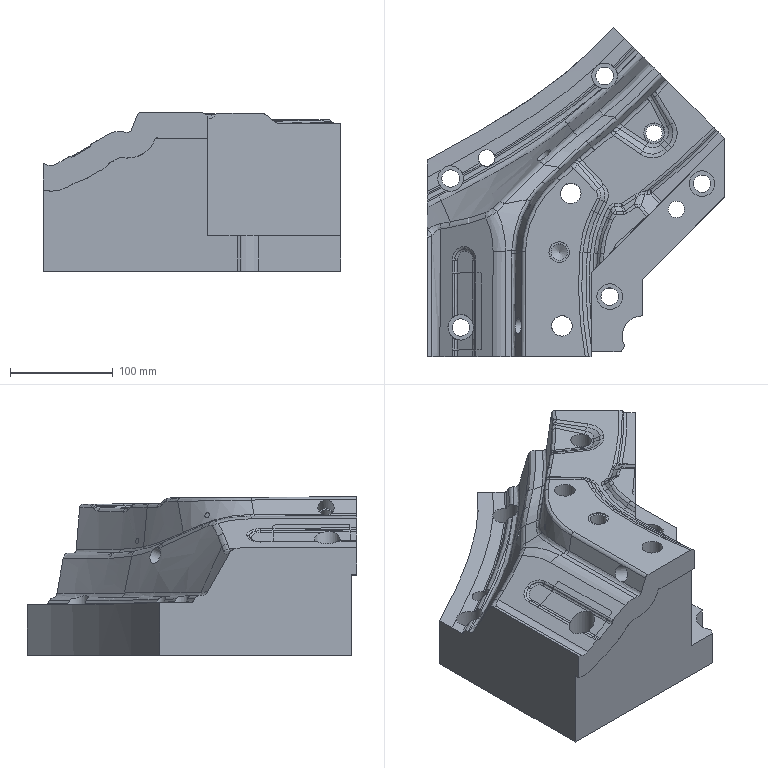Part | NX | features solid 2 | 1 solid | 227 faces | box 290.247 x 320.991 x 154.565 mm | volume 6396586 mm3 | spline 180 | cylinder 24 | plane 22 | cone 1 | commonest cylinder face diameters 16 x6 17 x5 25 x5 20 x4 13 x2 23 x1